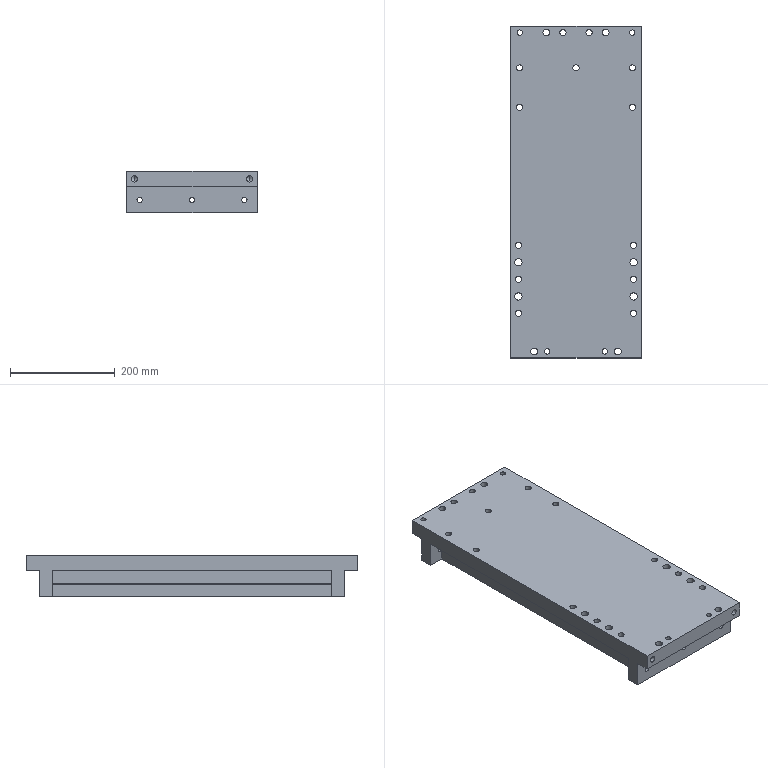Part | STEP file | MAT BAN KHONG LOGO | 1 solid | 102 faces | box 250 x 633.6 x 80 mm | volume 6062488 mm3 | cylinder 68 | plane 26 | cone 8 | commonest cylinder face diameters 11.835 x34 10.106 x18 13 x8 14 x8